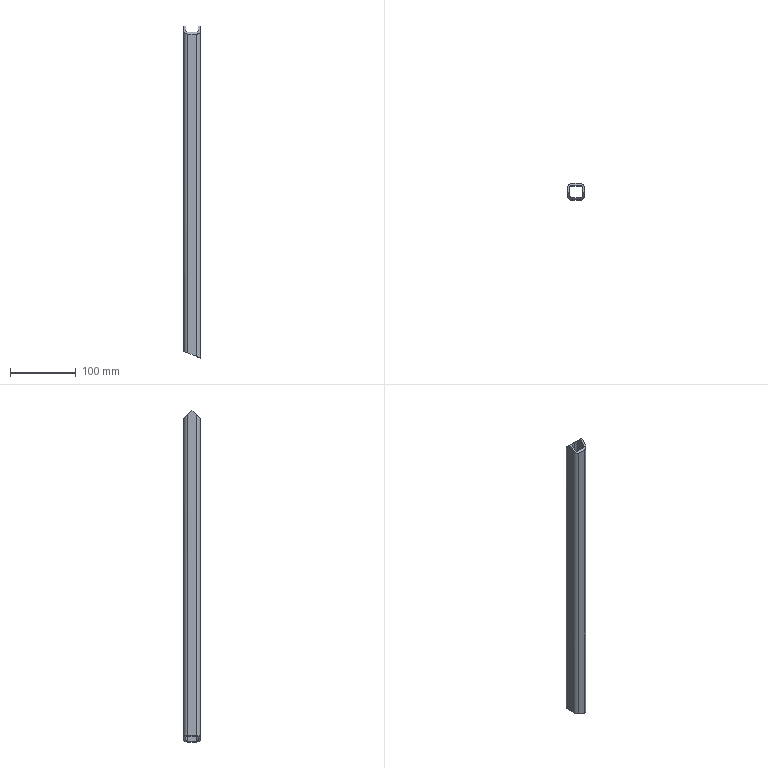Part | STEP file | ISO 10799-2 25x25x3 1784907954226 | 1 solid | 19 faces | box 25 x 25 x 504.794 mm | volume 118438 mm3 | plane 11 | cylinder 8 | commonest cylinder face diameters 6 x4 12 x4
STEP:
#1=CARTESIAN_POINT('',(12.5,6.5,-5.036));
#2=VERTEX_POINT('',#1);
#3=CARTESIAN_POINT('',(12.5,-6.5,-5.036));
#4=VERTEX_POINT('',#3);
#5=CARTESIAN_POINT('',(12.5,3.25,-5.036));
#6=DIRECTION('',(0.,-1.,0.));
#7=VECTOR('',#6,10.);
#8=LINE('',#5,#7);
#9=EDGE_CURVE('',#2,#4,#8,.T.);
#10=ORIENTED_EDGE('',*,*,#9,.T.);
#11=CARTESIAN_POINT('',(6.5,-12.5,-2.619));
#12=VERTEX_POINT('',#11);
#13=CARTESIAN_POINT('',(6.5,-6.5,-2.619));
#14=DIRECTION('',(0.3737,0.,0.9275));
#15=DIRECTION('',(-0.9275,0.,0.3737));
#16=AXIS2_PLACEMENT_3D('',#13,#14,#15);
#17=ELLIPSE('',#16,6.469,6.);
#18=EDGE_CURVE('',#12,#4,#17,.T.);
#19=ORIENTED_EDGE('',*,*,#18,.F.);
#20=CARTESIAN_POINT('',(-6.5,-12.5,2.619));
#21=VERTEX_POINT('',#20);
#22=CARTESIAN_POINT('',(2.796,-12.5,-1.127));
#23=DIRECTION('',(0.9275,0.,-0.3737));
#24=VECTOR('',#23,10.);
#25=LINE('',#22,#24);
#26=EDGE_CURVE('',#21,#12,#25,.T.);
#27=ORIENTED_EDGE('',*,*,#26,.F.);
#28=CARTESIAN_POINT('',(-12.5,-6.5,5.036));
#29=VERTEX_POINT('',#28);
#30=CARTESIAN_POINT('',(-6.5,-6.5,2.619));
#31=DIRECTION('',(0.3737,0.,0.9275));
#32=DIRECTION('',(0.9275,0.,-0.3737));
#33=AXIS2_PLACEMENT_3D('',#30,#31,#32);
#34=ELLIPSE('',#33,6.469,6.);
#35=EDGE_CURVE('',#29,#21,#34,.T.);
#36=ORIENTED_EDGE('',*,*,#35,.F.);
#37=CARTESIAN_POINT('',(-12.5,6.5,5.036));
#38=VERTEX_POINT('',#37);
#39=CARTESIAN_POINT('',(-12.5,-3.25,5.036));
#40=DIRECTION('',(0.,-1.,0.));
#41=VECTOR('',#40,10.);
#42=LINE('',#39,#41);
#43=EDGE_CURVE('',#38,#29,#42,.T.);
#44=ORIENTED_EDGE('',*,*,#43,.F.);
#45=CARTESIAN_POINT('',(-6.5,12.5,2.619));
#46=VERTEX_POINT('',#45);
#47=CARTESIAN_POINT('',(-6.5,6.5,2.619));
#48=DIRECTION('',(0.3737,0.,0.9275));
#49=DIRECTION('',(0.9275,0.,-0.3737));
#50=AXIS2_PLACEMENT_3D('',#47,#48,#49);
#51=ELLIPSE('',#50,6.469,6.);
#52=EDGE_CURVE('',#46,#38,#51,.T.);
#53=ORIENTED_EDGE('',*,*,#52,.F.);
#54=CARTESIAN_POINT('',(6.5,12.5,-2.619));
#55=VERTEX_POINT('',#54);
#56=CARTESIAN_POINT('',(-2.796,12.5,1.127));
#57=DIRECTION('',(-0.9275,0.,0.3737));
#58=VECTOR('',#57,10.);
#59=LINE('',#56,#58);
#60=EDGE_CURVE('',#55,#46,#59,.T.);
#61=ORIENTED_EDGE('',*,*,#60,.F.);
#62=CARTESIAN_POINT('',(6.5,6.5,-2.619));
#63=DIRECTION('',(0.3737,0.,0.9275));
#64=DIRECTION('',(-0.9275,0.,0.3737));
#65=AXIS2_PLACEMENT_3D('',#62,#63,#64);
#66=ELLIPSE('',#65,6.469,6.);
#67=EDGE_CURVE('',#2,#55,#66,.T.);
#68=ORIENTED_EDGE('',*,*,#67,.F.);
#69=EDGE_LOOP('',(#10,#19,#27,#36,#44,#53,#61,#68));
#70=FACE_OUTER_BOUND('',#69,.T.);
#71=CARTESIAN_POINT('',(9.5,6.5,-3.828));
#72=VERTEX_POINT('',#71);
#73=CARTESIAN_POINT('',(9.5,-6.5,-3.828));
#74=VERTEX_POINT('',#73);
#75=CARTESIAN_POINT('',(9.5,3.25,-3.828));
#76=DIRECTION('',(0.,-1.,0.));
#77=VECTOR('',#76,10.);
#78=LINE('',#75,#77);
#79=EDGE_CURVE('',#72,#74,#78,.T.);
#80=ORIENTED_EDGE('',*,*,#79,.F.);
#81=CARTESIAN_POINT('',(6.5,9.5,-2.619));
#82=VERTEX_POINT('',#81);
#83=CARTESIAN_POINT('',(6.5,6.5,-2.619));
#84=DIRECTION('',(-0.3737,0.,-0.9275));
#85=DIRECTION('',(-0.9275,0.,0.3737));
#86=AXIS2_PLACEMENT_3D('',#83,#84,#85);
#87=ELLIPSE('',#86,3.234,3.);
#88=EDGE_CURVE('',#82,#72,#87,.T.);
#89=ORIENTED_EDGE('',*,*,#88,.F.);
#90=CARTESIAN_POINT('',(-6.5,9.5,2.619));
#91=VERTEX_POINT('',#90);
#92=CARTESIAN_POINT('',(-2.796,9.5,1.127));
#93=DIRECTION('',(0.9275,0.,-0.3737));
#94=VECTOR('',#93,10.);
#95=LINE('',#92,#94);
#96=EDGE_CURVE('',#91,#82,#95,.T.);
#97=ORIENTED_EDGE('',*,*,#96,.F.);
#98=CARTESIAN_POINT('',(-9.5,6.5,3.828));
#99=VERTEX_POINT('',#98);
#100=CARTESIAN_POINT('',(-6.5,6.5,2.619));
#101=DIRECTION('',(-0.3737,0.,-0.9275));
#102=DIRECTION('',(0.9275,0.,-0.3737));
#103=AXIS2_PLACEMENT_3D('',#100,#101,#102);
#104=ELLIPSE('',#103,3.234,3.);
#105=EDGE_CURVE('',#99,#91,#104,.T.);
#106=ORIENTED_EDGE('',*,*,#105,.F.);
#107=CARTESIAN_POINT('',(-9.5,-6.5,3.828));
#108=VERTEX_POINT('',#107);
#109=CARTESIAN_POINT('',(-9.5,-3.25,3.828));
#110=DIRECTION('',(0.,1.,0.));
#111=VECTOR('',#110,10.);
#112=LINE('',#109,#111);
#113=EDGE_CURVE('',#108,#99,#112,.T.);
#114=ORIENTED_EDGE('',*,*,#113,.F.);
#115=CARTESIAN_POINT('',(-6.5,-9.5,2.619));
#116=VERTEX_POINT('',#115);
#117=CARTESIAN_POINT('',(-6.5,-6.5,2.619));
#118=DIRECTION('',(-0.3737,0.,-0.9275));
#119=DIRECTION('',(0.9275,0.,-0.3737));
#120=AXIS2_PLACEMENT_3D('',#117,#118,#119);
#121=ELLIPSE('',#120,3.234,3.);
#122=EDGE_CURVE('',#116,#108,#121,.T.);
#123=ORIENTED_EDGE('',*,*,#122,.F.);
#124=CARTESIAN_POINT('',(6.5,-9.5,-2.619));
#125=VERTEX_POINT('',#124);
#126=CARTESIAN_POINT('',(2.796,-9.5,-1.127));
#127=DIRECTION('',(-0.9275,0.,0.3737));
#128=VECTOR('',#127,10.);
#129=LINE('',#126,#128);
#130=EDGE_CURVE('',#125,#116,#129,.T.);
#131=ORIENTED_EDGE('',*,*,#130,.F.);
#132=CARTESIAN_POINT('',(6.5,-6.5,-2.619));
#133=DIRECTION('',(-0.3737,0.,-0.9275));
#134=DIRECTION('',(-0.9275,0.,0.3737));
#135=AXIS2_PLACEMENT_3D('',#132,#133,#134);
#136=ELLIPSE('',#135,3.234,3.);
#137=EDGE_CURVE('',#74,#125,#136,.T.);
#138=ORIENTED_EDGE('',*,*,#137,.F.);
#139=EDGE_LOOP('',(#80,#89,#97,#106,#114,#123,#131,#138));
#140=FACE_BOUND('',#139,.T.);
#141=CARTESIAN_POINT('',(0.,0.,0.));
#142=DIRECTION('',(0.3737,0.,0.9275));
#143=DIRECTION('',(0.9275,0.,-0.3737));
#144=AXIS2_PLACEMENT_3D('',#141,#142,#143);
#145=PLANE('',#144);
#146=ADVANCED_FACE('',(#70,#140),#145,.F.);
#147=ORIENTED_EDGE('',*,*,#113,.T.);
#148=CARTESIAN_POINT('',(-9.5,6.5,493.258));
#149=VERTEX_POINT('',#148);
#150=CARTESIAN_POINT('',(-9.5,6.5,0.));
#151=DIRECTION('',(0.,0.,1.));
#152=VECTOR('',#151,10.);
#153=LINE('',#150,#152);
#154=EDGE_CURVE('',#99,#149,#153,.T.);
#155=ORIENTED_EDGE('',*,*,#154,.T.);
#156=CARTESIAN_POINT('',(-9.5,0.000000002,499.758));
#157=VERTEX_POINT('',#156);
#158=CARTESIAN_POINT('',(-9.5,248.254,251.504));
#159=DIRECTION('',(0.,-0.7071,0.7071));
#160=VECTOR('',#159,10.);
#161=LINE('',#158,#160);
#162=EDGE_CURVE('',#149,#157,#161,.T.);
#163=ORIENTED_EDGE('',*,*,#162,.T.);
#164=CARTESIAN_POINT('',(-9.5,-6.5,493.258));
#165=VERTEX_POINT('',#164);
#166=CARTESIAN_POINT('',(-9.5,-251.504,248.254));
#167=DIRECTION('',(0.,-0.7071,-0.7071));
#168=VECTOR('',#167,10.);
#169=LINE('',#166,#168);
#170=EDGE_CURVE('',#157,#165,#169,.T.);
#171=ORIENTED_EDGE('',*,*,#170,.T.);
#172=CARTESIAN_POINT('',(-9.5,-6.5,0.));
#173=DIRECTION('',(0.,0.,-1.));
#174=VECTOR('',#173,10.);
#175=LINE('',#172,#174);
#176=EDGE_CURVE('',#165,#108,#175,.T.);
#177=ORIENTED_EDGE('',*,*,#176,.T.);
#178=EDGE_LOOP('',(#147,#155,#163,#171,#177));
#179=FACE_OUTER_BOUND('',#178,.T.);
#180=CARTESIAN_POINT('',(-9.5,-6.5,0.));
#181=DIRECTION('',(-1.,0.,0.));
#182=DIRECTION('',(0.,0.,1.));
#183=AXIS2_PLACEMENT_3D('',#180,#181,#182);
#184=PLANE('',#183);
#185=ADVANCED_FACE('',(#179),#184,.F.);
#186=ORIENTED_EDGE('',*,*,#105,.T.);
#187=CARTESIAN_POINT('',(-6.5,9.5,490.258));
#188=VERTEX_POINT('',#187);
#189=CARTESIAN_POINT('',(-6.5,9.5,0.));
#190=DIRECTION('',(0.,0.,-1.));
#191=VECTOR('',#190,10.);
#192=LINE('',#189,#191);
#193=EDGE_CURVE('',#188,#91,#192,.T.);
#194=ORIENTED_EDGE('',*,*,#193,.F.);
#195=CARTESIAN_POINT('',(-6.5,6.5,493.258));
#196=DIRECTION('',(0.,0.7071,0.7071));
#197=DIRECTION('',(0.,-0.7071,0.7071));
#198=AXIS2_PLACEMENT_3D('',#195,#196,#197);
#199=ELLIPSE('',#198,4.243,3.);
#200=EDGE_CURVE('',#188,#149,#199,.T.);
#201=ORIENTED_EDGE('',*,*,#200,.T.);
#202=ORIENTED_EDGE('',*,*,#154,.F.);
#203=EDGE_LOOP('',(#186,#194,#201,#202));
#204=FACE_OUTER_BOUND('',#203,.T.);
#205=CARTESIAN_POINT('',(-6.5,6.5,0.));
#206=DIRECTION('',(0.,0.,1.));
#207=DIRECTION('',(0.,-1.,0.));
#208=AXIS2_PLACEMENT_3D('',#205,#206,#207);
#209=CYLINDRICAL_SURFACE('',#208,3.);
#210=ADVANCED_FACE('',(#204),#209,.F.);
#211=ORIENTED_EDGE('',*,*,#96,.T.);
#212=CARTESIAN_POINT('',(6.5,9.5,490.258));
#213=VERTEX_POINT('',#212);
#214=CARTESIAN_POINT('',(6.5,9.5,0.));
#215=DIRECTION('',(0.,0.,-1.));
#216=VECTOR('',#215,10.);
#217=LINE('',#214,#216);
#218=EDGE_CURVE('',#213,#82,#217,.T.);
#219=ORIENTED_EDGE('',*,*,#218,.F.);
#220=CARTESIAN_POINT('',(-3.25,9.5,490.258));
#221=DIRECTION('',(-1.,0.,0.));
#222=VECTOR('',#221,10.);
#223=LINE('',#220,#222);
#224=EDGE_CURVE('',#213,#188,#223,.T.);
#225=ORIENTED_EDGE('',*,*,#224,.T.);
#226=ORIENTED_EDGE('',*,*,#193,.T.);
#227=EDGE_LOOP('',(#211,#219,#225,#226));
#228=FACE_OUTER_BOUND('',#227,.T.);
#229=CARTESIAN_POINT('',(-6.5,9.5,0.));
#230=DIRECTION('',(0.,1.,0.));
#231=DIRECTION('',(0.,0.,1.));
#232=AXIS2_PLACEMENT_3D('',#229,#230,#231);
#233=PLANE('',#232);
#234=ADVANCED_FACE('',(#228),#233,.F.);
#235=ORIENTED_EDGE('',*,*,#88,.T.);
#236=CARTESIAN_POINT('',(9.5,6.5,493.258));
#237=VERTEX_POINT('',#236);
#238=CARTESIAN_POINT('',(9.5,6.5,0.));
#239=DIRECTION('',(0.,0.,-1.));
#240=VECTOR('',#239,10.);
#241=LINE('',#238,#240);
#242=EDGE_CURVE('',#237,#72,#241,.T.);
#243=ORIENTED_EDGE('',*,*,#242,.F.);
#244=CARTESIAN_POINT('',(6.5,6.5,493.258));
#245=DIRECTION('',(0.,0.7071,0.7071));
#246=DIRECTION('',(0.,-0.7071,0.7071));
#247=AXIS2_PLACEMENT_3D('',#244,#245,#246);
#248=ELLIPSE('',#247,4.243,3.);
#249=EDGE_CURVE('',#237,#213,#248,.T.);
#250=ORIENTED_EDGE('',*,*,#249,.T.);
#251=ORIENTED_EDGE('',*,*,#218,.T.);
#252=EDGE_LOOP('',(#235,#243,#250,#251));
#253=FACE_OUTER_BOUND('',#252,.T.);
#254=CARTESIAN_POINT('',(6.5,6.5,0.));
#255=DIRECTION('',(0.,0.,1.));
#256=DIRECTION('',(-1.,0.,0.));
#257=AXIS2_PLACEMENT_3D('',#254,#255,#256);
#258=CYLINDRICAL_SURFACE('',#257,3.);
#259=ADVANCED_FACE('',(#253),#258,.F.);
#260=ORIENTED_EDGE('',*,*,#43,.T.);
#261=CARTESIAN_POINT('',(-12.5,-6.5,493.258));
#262=VERTEX_POINT('',#261);
#263=CARTESIAN_POINT('',(-12.5,-6.5,0.));
#264=DIRECTION('',(0.,0.,-1.));
#265=VECTOR('',#264,10.);
#266=LINE('',#263,#265);
#267=EDGE_CURVE('',#262,#29,#266,.T.);
#268=ORIENTED_EDGE('',*,*,#267,.F.);
#269=CARTESIAN_POINT('',(-12.5,0.000000002,499.758));
#270=VERTEX_POINT('',#269);
#271=CARTESIAN_POINT('',(-12.5,-251.504,248.254));
#272=DIRECTION('',(0.,0.7071,0.7071));
#273=VECTOR('',#272,10.);
#274=LINE('',#271,#273);
#275=EDGE_CURVE('',#262,#270,#274,.T.);
#276=ORIENTED_EDGE('',*,*,#275,.T.);
#277=CARTESIAN_POINT('',(-12.5,6.5,493.258));
#278=VERTEX_POINT('',#277);
#279=CARTESIAN_POINT('',(-12.5,248.254,251.504));
#280=DIRECTION('',(0.,0.7071,-0.7071));
#281=VECTOR('',#280,10.);
#282=LINE('',#279,#281);
#283=EDGE_CURVE('',#270,#278,#282,.T.);
#284=ORIENTED_EDGE('',*,*,#283,.T.);
#285=CARTESIAN_POINT('',(-12.5,6.5,0.));
#286=DIRECTION('',(0.,0.,-1.));
#287=VECTOR('',#286,10.);
#288=LINE('',#285,#287);
#289=EDGE_CURVE('',#278,#38,#288,.T.);
#290=ORIENTED_EDGE('',*,*,#289,.T.);
#291=EDGE_LOOP('',(#260,#268,#276,#284,#290));
#292=FACE_OUTER_BOUND('',#291,.T.);
#293=CARTESIAN_POINT('',(-12.5,-6.5,0.));
#294=DIRECTION('',(-1.,0.,0.));
#295=DIRECTION('',(0.,0.,1.));
#296=AXIS2_PLACEMENT_3D('',#293,#294,#295);
#297=PLANE('',#296);
#298=ADVANCED_FACE('',(#292),#297,.T.);
#299=ORIENTED_EDGE('',*,*,#35,.T.);
#300=CARTESIAN_POINT('',(-6.5,-12.5,487.258));
#301=VERTEX_POINT('',#300);
#302=CARTESIAN_POINT('',(-6.5,-12.5,0.));
#303=DIRECTION('',(0.,0.,1.));
#304=VECTOR('',#303,10.);
#305=LINE('',#302,#304);
#306=EDGE_CURVE('',#21,#301,#305,.T.);
#307=ORIENTED_EDGE('',*,*,#306,.T.);
#308=CARTESIAN_POINT('',(-6.5,-6.5,493.258));
#309=DIRECTION('',(0.,0.7071,-0.7071));
#310=DIRECTION('',(0.,0.7071,0.7071));
#311=AXIS2_PLACEMENT_3D('',#308,#309,#310);
#312=ELLIPSE('',#311,8.485,6.);
#313=EDGE_CURVE('',#301,#262,#312,.T.);
#314=ORIENTED_EDGE('',*,*,#313,.T.);
#315=ORIENTED_EDGE('',*,*,#267,.T.);
#316=EDGE_LOOP('',(#299,#307,#314,#315));
#317=FACE_OUTER_BOUND('',#316,.T.);
#318=CARTESIAN_POINT('',(-6.5,-6.5,0.));
#319=DIRECTION('',(0.,0.,1.));
#320=DIRECTION('',(1.,0.,0.));
#321=AXIS2_PLACEMENT_3D('',#318,#319,#320);
#322=CYLINDRICAL_SURFACE('',#321,6.);
#323=ADVANCED_FACE('',(#317),#322,.T.);
#324=ORIENTED_EDGE('',*,*,#26,.T.);
#325=CARTESIAN_POINT('',(6.5,-12.5,487.258));
#326=VERTEX_POINT('',#325);
#327=CARTESIAN_POINT('',(6.5,-12.5,0.));
#328=DIRECTION('',(0.,0.,-1.));
#329=VECTOR('',#328,10.);
#330=LINE('',#327,#329);
#331=EDGE_CURVE('',#326,#12,#330,.T.);
#332=ORIENTED_EDGE('',*,*,#331,.F.);
#333=CARTESIAN_POINT('',(3.25,-12.5,487.258));
#334=DIRECTION('',(-1.,0.,0.));
#335=VECTOR('',#334,10.);
#336=LINE('',#333,#335);
#337=EDGE_CURVE('',#326,#301,#336,.T.);
#338=ORIENTED_EDGE('',*,*,#337,.T.);
#339=ORIENTED_EDGE('',*,*,#306,.F.);
#340=EDGE_LOOP('',(#324,#332,#338,#339));
#341=FACE_OUTER_BOUND('',#340,.T.);
#342=CARTESIAN_POINT('',(6.5,-12.5,0.));
#343=DIRECTION('',(0.,-1.,0.));
#344=DIRECTION('',(0.,0.,-1.));
#345=AXIS2_PLACEMENT_3D('',#342,#343,#344);
#346=PLANE('',#345);
#347=ADVANCED_FACE('',(#341),#346,.T.);
#348=ORIENTED_EDGE('',*,*,#18,.T.);
#349=CARTESIAN_POINT('',(12.5,-6.5,493.258));
#350=VERTEX_POINT('',#349);
#351=CARTESIAN_POINT('',(12.5,-6.5,0.));
#352=DIRECTION('',(0.,0.,-1.));
#353=VECTOR('',#352,10.);
#354=LINE('',#351,#353);
#355=EDGE_CURVE('',#350,#4,#354,.T.);
#356=ORIENTED_EDGE('',*,*,#355,.F.);
#357=CARTESIAN_POINT('',(6.5,-6.5,493.258));
#358=DIRECTION('',(0.,0.7071,-0.7071));
#359=DIRECTION('',(0.,0.7071,0.7071));
#360=AXIS2_PLACEMENT_3D('',#357,#358,#359);
#361=ELLIPSE('',#360,8.485,6.);
#362=EDGE_CURVE('',#350,#326,#361,.T.);
#363=ORIENTED_EDGE('',*,*,#362,.T.);
#364=ORIENTED_EDGE('',*,*,#331,.T.);
#365=EDGE_LOOP('',(#348,#356,#363,#364));
#366=FACE_OUTER_BOUND('',#365,.T.);
#367=CARTESIAN_POINT('',(6.5,-6.5,0.));
#368=DIRECTION('',(0.,0.,1.));
#369=DIRECTION('',(0.,1.,0.));
#370=AXIS2_PLACEMENT_3D('',#367,#368,#369);
#371=CYLINDRICAL_SURFACE('',#370,6.);
#372=ADVANCED_FACE('',(#366),#371,.T.);
#373=CARTESIAN_POINT('',(0.,0.000000002,499.758));
#374=DIRECTION('',(1.,0.,0.));
#375=VECTOR('',#374,10.);
#376=LINE('',#373,#375);
#377=EDGE_CURVE('',#270,#157,#376,.T.);
#378=ORIENTED_EDGE('',*,*,#377,.T.);
#379=ORIENTED_EDGE('',*,*,#162,.F.);
#380=ORIENTED_EDGE('',*,*,#200,.F.);
#381=ORIENTED_EDGE('',*,*,#224,.F.);
#382=ORIENTED_EDGE('',*,*,#249,.F.);
#383=CARTESIAN_POINT('',(9.5,0.000000002,499.758));
#384=VERTEX_POINT('',#383);
#385=CARTESIAN_POINT('',(9.5,251.504,248.254));
#386=DIRECTION('',(0.,0.7071,-0.7071));
#387=VECTOR('',#386,10.);
#388=LINE('',#385,#387);
#389=EDGE_CURVE('',#384,#237,#388,.T.);
#390=ORIENTED_EDGE('',*,*,#389,.F.);
#391=CARTESIAN_POINT('',(12.5,0.000000002,499.758));
#392=VERTEX_POINT('',#391);
#393=CARTESIAN_POINT('',(0.,0.000000002,499.758));
#394=DIRECTION('',(1.,0.,0.));
#395=VECTOR('',#394,10.);
#396=LINE('',#393,#395);
#397=EDGE_CURVE('',#384,#392,#396,.T.);
#398=ORIENTED_EDGE('',*,*,#397,.T.);
#399=CARTESIAN_POINT('',(12.5,6.5,493.258));
#400=VERTEX_POINT('',#399);
#401=CARTESIAN_POINT('',(12.5,251.504,248.254));
#402=DIRECTION('',(0.,-0.7071,0.7071));
#403=VECTOR('',#402,10.);
#404=LINE('',#401,#403);
#405=EDGE_CURVE('',#400,#392,#404,.T.);
#406=ORIENTED_EDGE('',*,*,#405,.F.);
#407=CARTESIAN_POINT('',(6.5,12.5,487.258));
#408=VERTEX_POINT('',#407);
#409=CARTESIAN_POINT('',(6.5,6.5,493.258));
#410=DIRECTION('',(0.,-0.7071,-0.7071));
#411=DIRECTION('',(0.,-0.7071,0.7071));
#412=AXIS2_PLACEMENT_3D('',#409,#410,#411);
#413=ELLIPSE('',#412,8.485,6.);
#414=EDGE_CURVE('',#408,#400,#413,.T.);
#415=ORIENTED_EDGE('',*,*,#414,.F.);
#416=CARTESIAN_POINT('',(-6.5,12.5,487.258));
#417=VERTEX_POINT('',#416);
#418=CARTESIAN_POINT('',(-3.25,12.5,487.258));
#419=DIRECTION('',(1.,0.,0.));
#420=VECTOR('',#419,10.);
#421=LINE('',#418,#420);
#422=EDGE_CURVE('',#417,#408,#421,.T.);
#423=ORIENTED_EDGE('',*,*,#422,.F.);
#424=CARTESIAN_POINT('',(-6.5,6.5,493.258));
#425=DIRECTION('',(0.,-0.7071,-0.7071));
#426=DIRECTION('',(0.,-0.7071,0.7071));
#427=AXIS2_PLACEMENT_3D('',#424,#425,#426);
#428=ELLIPSE('',#427,8.485,6.);
#429=EDGE_CURVE('',#278,#417,#428,.T.);
#430=ORIENTED_EDGE('',*,*,#429,.F.);
#431=ORIENTED_EDGE('',*,*,#283,.F.);
#432=EDGE_LOOP('',(#378,#379,#380,#381,#382,#390,#398,#406,#415,#423,#430,#431));
#433=FACE_OUTER_BOUND('',#432,.T.);
#434=CARTESIAN_POINT('',(0.,249.879,249.879));
#435=DIRECTION('',(0.,-0.7071,-0.7071));
#436=DIRECTION('',(-1.,0.,0.));
#437=AXIS2_PLACEMENT_3D('',#434,#435,#436);
#438=PLANE('',#437);
#439=ADVANCED_FACE('',(#433),#438,.F.);
#440=ORIENTED_EDGE('',*,*,#79,.T.);
#441=CARTESIAN_POINT('',(9.5,-6.5,493.258));
#442=VERTEX_POINT('',#441);
#443=CARTESIAN_POINT('',(9.5,-6.5,0.));
#444=DIRECTION('',(0.,0.,-1.));
#445=VECTOR('',#444,10.);
#446=LINE('',#443,#445);
#447=EDGE_CURVE('',#442,#74,#446,.T.);
#448=ORIENTED_EDGE('',*,*,#447,.F.);
#449=CARTESIAN_POINT('',(9.5,-248.254,251.504));
#450=DIRECTION('',(0.,0.7071,0.7071));
#451=VECTOR('',#450,10.);
#452=LINE('',#449,#451);
#453=EDGE_CURVE('',#442,#384,#452,.T.);
#454=ORIENTED_EDGE('',*,*,#453,.T.);
#455=ORIENTED_EDGE('',*,*,#389,.T.);
#456=ORIENTED_EDGE('',*,*,#242,.T.);
#457=EDGE_LOOP('',(#440,#448,#454,#455,#456));
#458=FACE_OUTER_BOUND('',#457,.T.);
#459=CARTESIAN_POINT('',(9.5,6.5,0.));
#460=DIRECTION('',(1.,0.,0.));
#461=DIRECTION('',(0.,0.,-1.));
#462=AXIS2_PLACEMENT_3D('',#459,#460,#461);
#463=PLANE('',#462);
#464=ADVANCED_FACE('',(#458),#463,.F.);
#465=CARTESIAN_POINT('',(12.5,-248.254,251.504));
#466=DIRECTION('',(0.,-0.7071,-0.7071));
#467=VECTOR('',#466,10.);
#468=LINE('',#465,#467);
#469=EDGE_CURVE('',#392,#350,#468,.T.);
#470=ORIENTED_EDGE('',*,*,#469,.F.);
#471=ORIENTED_EDGE('',*,*,#397,.F.);
#472=ORIENTED_EDGE('',*,*,#453,.F.);
#473=CARTESIAN_POINT('',(6.5,-9.5,490.258));
#474=VERTEX_POINT('',#473);
#475=CARTESIAN_POINT('',(6.5,-6.5,493.258));
#476=DIRECTION('',(0.,-0.7071,0.7071));
#477=DIRECTION('',(0.,0.7071,0.7071));
#478=AXIS2_PLACEMENT_3D('',#475,#476,#477);
#479=ELLIPSE('',#478,4.243,3.);
#480=EDGE_CURVE('',#474,#442,#479,.T.);
#481=ORIENTED_EDGE('',*,*,#480,.F.);
#482=CARTESIAN_POINT('',(-6.5,-9.5,490.258));
#483=VERTEX_POINT('',#482);
#484=CARTESIAN_POINT('',(3.25,-9.5,490.258));
#485=DIRECTION('',(1.,0.,0.));
#486=VECTOR('',#485,10.);
#487=LINE('',#484,#486);
#488=EDGE_CURVE('',#483,#474,#487,.T.);
#489=ORIENTED_EDGE('',*,*,#488,.F.);
#490=CARTESIAN_POINT('',(-6.5,-6.5,493.258));
#491=DIRECTION('',(0.,-0.7071,0.7071));
#492=DIRECTION('',(0.,0.7071,0.7071));
#493=AXIS2_PLACEMENT_3D('',#490,#491,#492);
#494=ELLIPSE('',#493,4.243,3.);
#495=EDGE_CURVE('',#165,#483,#494,.T.);
#496=ORIENTED_EDGE('',*,*,#495,.F.);
#497=ORIENTED_EDGE('',*,*,#170,.F.);
#498=ORIENTED_EDGE('',*,*,#377,.F.);
#499=ORIENTED_EDGE('',*,*,#275,.F.);
#500=ORIENTED_EDGE('',*,*,#313,.F.);
#501=ORIENTED_EDGE('',*,*,#337,.F.);
#502=ORIENTED_EDGE('',*,*,#362,.F.);
#503=EDGE_LOOP('',(#470,#471,#472,#481,#489,#496,#497,#498,#499,#500,#501,#502));
#504=FACE_OUTER_BOUND('',#503,.T.);
#505=CARTESIAN_POINT('',(0.,-249.879,249.879));
#506=DIRECTION('',(0.,0.7071,-0.7071));
#507=DIRECTION('',(-1.,0.,0.));
#508=AXIS2_PLACEMENT_3D('',#505,#506,#507);
#509=PLANE('',#508);
#510=ADVANCED_FACE('',(#504),#509,.F.);
#511=ORIENTED_EDGE('',*,*,#122,.T.);
#512=ORIENTED_EDGE('',*,*,#176,.F.);
#513=ORIENTED_EDGE('',*,*,#495,.T.);
#514=CARTESIAN_POINT('',(-6.5,-9.5,0.));
#515=DIRECTION('',(0.,0.,-1.));
#516=VECTOR('',#515,10.);
#517=LINE('',#514,#516);
#518=EDGE_CURVE('',#483,#116,#517,.T.);
#519=ORIENTED_EDGE('',*,*,#518,.T.);
#520=EDGE_LOOP('',(#511,#512,#513,#519));
#521=FACE_OUTER_BOUND('',#520,.T.);
#522=CARTESIAN_POINT('',(-6.5,-6.5,0.));
#523=DIRECTION('',(0.,0.,1.));
#524=DIRECTION('',(1.,0.,0.));
#525=AXIS2_PLACEMENT_3D('',#522,#523,#524);
#526=CYLINDRICAL_SURFACE('',#525,3.);
#527=ADVANCED_FACE('',(#521),#526,.F.);
#528=ORIENTED_EDGE('',*,*,#130,.T.);
#529=ORIENTED_EDGE('',*,*,#518,.F.);
#530=ORIENTED_EDGE('',*,*,#488,.T.);
#531=CARTESIAN_POINT('',(6.5,-9.5,0.));
#532=DIRECTION('',(0.,0.,-1.));
#533=VECTOR('',#532,10.);
#534=LINE('',#531,#533);
#535=EDGE_CURVE('',#474,#125,#534,.T.);
#536=ORIENTED_EDGE('',*,*,#535,.T.);
#537=EDGE_LOOP('',(#528,#529,#530,#536));
#538=FACE_OUTER_BOUND('',#537,.T.);
#539=CARTESIAN_POINT('',(6.5,-9.5,0.));
#540=DIRECTION('',(0.,-1.,0.));
#541=DIRECTION('',(0.,0.,-1.));
#542=AXIS2_PLACEMENT_3D('',#539,#540,#541);
#543=PLANE('',#542);
#544=ADVANCED_FACE('',(#538),#543,.F.);
#545=ORIENTED_EDGE('',*,*,#137,.T.);
#546=ORIENTED_EDGE('',*,*,#535,.F.);
#547=ORIENTED_EDGE('',*,*,#480,.T.);
#548=ORIENTED_EDGE('',*,*,#447,.T.);
#549=EDGE_LOOP('',(#545,#546,#547,#548));
#550=FACE_OUTER_BOUND('',#549,.T.);
#551=CARTESIAN_POINT('',(6.5,-6.5,0.));
#552=DIRECTION('',(0.,0.,1.));
#553=DIRECTION('',(0.,1.,0.));
#554=AXIS2_PLACEMENT_3D('',#551,#552,#553);
#555=CYLINDRICAL_SURFACE('',#554,3.);
#556=ADVANCED_FACE('',(#550),#555,.F.);
#557=ORIENTED_EDGE('',*,*,#405,.T.);
#558=ORIENTED_EDGE('',*,*,#469,.T.);
#559=ORIENTED_EDGE('',*,*,#355,.T.);
#560=ORIENTED_EDGE('',*,*,#9,.F.);
#561=CARTESIAN_POINT('',(12.5,6.5,0.));
#562=DIRECTION('',(0.,0.,-1.));
#563=VECTOR('',#562,10.);
#564=LINE('',#561,#563);
#565=EDGE_CURVE('',#400,#2,#564,.T.);
#566=ORIENTED_EDGE('',*,*,#565,.F.);
#567=EDGE_LOOP('',(#557,#558,#559,#560,#566));
#568=FACE_OUTER_BOUND('',#567,.T.);
#569=CARTESIAN_POINT('',(12.5,6.5,0.));
#570=DIRECTION('',(1.,0.,0.));
#571=DIRECTION('',(0.,0.,-1.));
#572=AXIS2_PLACEMENT_3D('',#569,#570,#571);
#573=PLANE('',#572);
#574=ADVANCED_FACE('',(#568),#573,.T.);
#575=ORIENTED_EDGE('',*,*,#52,.T.);
#576=ORIENTED_EDGE('',*,*,#289,.F.);
#577=ORIENTED_EDGE('',*,*,#429,.T.);
#578=CARTESIAN_POINT('',(-6.5,12.5,0.));
#579=DIRECTION('',(0.,0.,-1.));
#580=VECTOR('',#579,10.);
#581=LINE('',#578,#580);
#582=EDGE_CURVE('',#417,#46,#581,.T.);
#583=ORIENTED_EDGE('',*,*,#582,.T.);
#584=EDGE_LOOP('',(#575,#576,#577,#583));
#585=FACE_OUTER_BOUND('',#584,.T.);
#586=CARTESIAN_POINT('',(-6.5,6.5,0.));
#587=DIRECTION('',(0.,0.,1.));
#588=DIRECTION('',(0.,-1.,0.));
#589=AXIS2_PLACEMENT_3D('',#586,#587,#588);
#590=CYLINDRICAL_SURFACE('',#589,6.);
#591=ADVANCED_FACE('',(#585),#590,.T.);
#592=ORIENTED_EDGE('',*,*,#60,.T.);
#593=ORIENTED_EDGE('',*,*,#582,.F.);
#594=ORIENTED_EDGE('',*,*,#422,.T.);
#595=CARTESIAN_POINT('',(6.5,12.5,0.));
#596=DIRECTION('',(0.,0.,-1.));
#597=VECTOR('',#596,10.);
#598=LINE('',#595,#597);
#599=EDGE_CURVE('',#408,#55,#598,.T.);
#600=ORIENTED_EDGE('',*,*,#599,.T.);
#601=EDGE_LOOP('',(#592,#593,#594,#600));
#602=FACE_OUTER_BOUND('',#601,.T.);
#603=CARTESIAN_POINT('',(-6.5,12.5,0.));
#604=DIRECTION('',(0.,1.,0.));
#605=DIRECTION('',(0.,0.,1.));
#606=AXIS2_PLACEMENT_3D('',#603,#604,#605);
#607=PLANE('',#606);
#608=ADVANCED_FACE('',(#602),#607,.T.);
#609=ORIENTED_EDGE('',*,*,#67,.T.);
#610=ORIENTED_EDGE('',*,*,#599,.F.);
#611=ORIENTED_EDGE('',*,*,#414,.T.);
#612=ORIENTED_EDGE('',*,*,#565,.T.);
#613=EDGE_LOOP('',(#609,#610,#611,#612));
#614=FACE_OUTER_BOUND('',#613,.T.);
#615=CARTESIAN_POINT('',(6.5,6.5,0.));
#616=DIRECTION('',(0.,0.,1.));
#617=DIRECTION('',(-1.,0.,0.));
#618=AXIS2_PLACEMENT_3D('',#615,#616,#617);
#619=CYLINDRICAL_SURFACE('',#618,6.);
#620=ADVANCED_FACE('',(#614),#619,.T.);
#621=CLOSED_SHELL('',(#146,#185,#210,#234,#259,#298,#323,#347,#372,#439,#464,#510,#527,#544,#556,#574,#591,#608,#620));
#622=MANIFOLD_SOLID_BREP('',#621);
#623=(LENGTH_UNIT()NAMED_UNIT(*)SI_UNIT(.MILLI.,.METRE.));
#624=UNCERTAINTY_MEASURE_WITH_UNIT(LENGTH_MEASURE(0.01),#623,'','');
#625=(NAMED_UNIT(*)PLANE_ANGLE_UNIT()SI_UNIT($,.RADIAN.));
#626=(NAMED_UNIT(*)SI_UNIT($,.STERADIAN.)SOLID_ANGLE_UNIT());
#627=(GEOMETRIC_REPRESENTATION_CONTEXT(3)GLOBAL_UNCERTAINTY_ASSIGNED_CONTEXT((#624))GLOBAL_UNIT_ASSIGNED_CONTEXT((#623,#625,#626))REPRESENTATION_CONTEXT('',''));
#628=ADVANCED_BREP_SHAPE_REPRESENTATION('',(#622),#627);